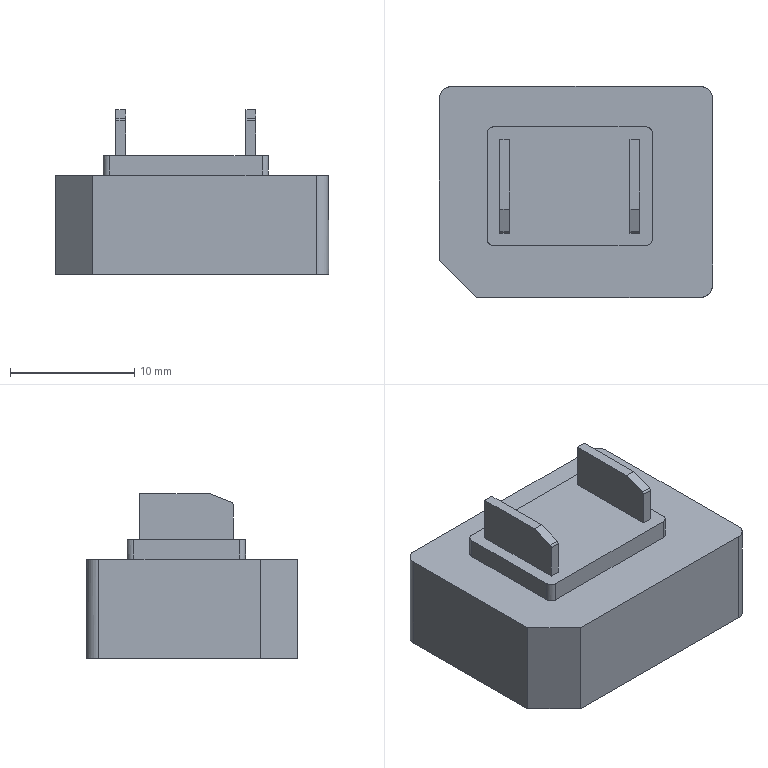NC program | PowerMill | posted by the shop | part box 22 x 17 x 13.286 mm
Lines 1 to 1591 of 53717:
%
G40 G49 G17 G80
( TOOL ID   D10C_1_1 )
( TOOL DIA. 10. TIP RAD 0 LENGTH 68.72 )
( Z = -.055 )
T1 M6
T2
G91 G28 Z0
G0 G90 G54
M08
S8000 M3
G0 X0 Y0 M8
G43 Z10.2 H1
X13.8 Y11.3
Z1.145
G1 Z-.055 F6000
X-13.8 F10000
Y5.65
X13.8
Y0
X-13.8
Y-5.65
X13.8
Y-11.3
X-13.8
X-18.8
G0 Z10.2
X-.5 Y.458
Z9.895
X19.223 Y5.979
Z.727
G1 Z-.473 F6000
X18.695 F10000
G3 X13.948 Y1.231 I0 J-4.748
G1 Y-11.112
G2 X12.948 Y-12.112 I-1. J0
G1 X-13.947
G2 X-14.947 Y-11.112 I0 J1.
G1 Y12.027
G2 X-13.947 Y13.027 I1. J0
G1 X12.948
G2 X13.948 Y12.027 I0 J-1.
G1 Y1.231
X10.448
Y-1.863
X10.42 Y-2.636
X10.293 Y-3.41
X10.051 Y-4.183
X9.942 Y-4.443
X9.671 Y-4.956
X9.168 Y-5.668
X8.395 Y-6.418
X7.621 Y-6.924
X6.796 Y-7.277
X6.075 Y-7.462
X5.301 Y-7.542
X4.528 Y-7.544
X3.754 Y-7.511
X2.981 Y-7.364
X2.207 Y-7.089
X1.434 Y-6.662
X1.212 Y-6.503
X.661 Y-6.033
X.378 Y-5.73
X-.099 Y-5.088
G3 X-.901 Y-5.088 I-.401 J-.298
G1 X-1.379 Y-5.73
X-1.66 Y-6.032
X-2.213 Y-6.503
X-2.433 Y-6.661
X-3.206 Y-7.088
X-3.98 Y-7.364
X-4.753 Y-7.511
X-5.527 Y-7.544
X-6.3 Y-7.542
X-7.074 Y-7.462
X-7.847 Y-7.261
X-8.62 Y-6.924
X-9.394 Y-6.418
X-10.114 Y-5.73
X-10.673 Y-4.956
X-10.941 Y-4.445
X-11.051 Y-4.183
X-11.294 Y-3.41
X-11.42 Y-2.636
X-11.448 Y-1.863
X-11.447 Y4.325
X-11.376 Y5.098
X-11.187 Y5.871
X-10.941 Y6.492
X-10.381 Y7.418
X-10.167 Y7.684
X-9.667 Y8.192
X-9.394 Y8.419
X-8.62 Y8.917
X-7.847 Y9.249
X-7.074 Y9.447
X-6.3 Y9.527
X-5.527 Y9.529
X-4.753 Y9.496
X-3.98 Y9.35
X-3.206 Y9.079
X-2.966 Y8.965
X-2.433 Y8.658
X-1.825 Y8.192
X-1.66 Y8.039
X-1.111 Y7.418
X-.91 Y7.13
G3 X-.09 Y7.13 I.41 J.286
G1 X.111 Y7.418
X.661 Y8.04
X.825 Y8.192
X1.434 Y8.658
X1.966 Y8.965
X2.207 Y9.079
X2.981 Y9.351
X3.754 Y9.496
X4.528 Y9.529
X5.301 Y9.527
X6.075 Y9.447
X6.848 Y9.249
X7.527 Y8.965
X8.395 Y8.418
X8.667 Y8.192
X9.168 Y7.683
X9.381 Y7.418
X9.865 Y6.645
X10.187 Y5.871
X10.376 Y5.098
X10.447 Y4.325
X10.448 Y1.231
X13.948
G0 Z3.36
G1 X19.223 Y5.979
G0 Z.36
G1 Z-.84 F6000
X18.695 F10000
G3 X13.948 Y1.231 I0 J-4.748
G1 Y-11.112
G2 X12.948 Y-12.112 I-1. J0
G1 X-13.947
G2 X-14.947 Y-11.112 I0 J1.
G1 Y12.027
G2 X-13.947 Y13.027 I1. J0
G1 X12.948
G2 X13.948 Y12.027 I0 J-1.
G1 Y2.497
X10.447 Y2.496
X10.448 Y.668
Y-1.863
Y-1.864
Y-2.636
X10.432 Y-3.41
X10.325 Y-4.183
X10.107 Y-4.956
X9.942 Y-5.36
X9.755 Y-5.73
X9.168 Y-6.582
X8.453 Y-7.277
X7.621 Y-7.834
X7.162 Y-8.05
X6.848 Y-8.161
X6.075 Y-8.362
X5.301 Y-8.448
X4.528 Y-8.45
X3.754 Y-8.413
X2.981 Y-8.27
X2.333 Y-8.05
X1.434 Y-7.566
X1.041 Y-7.277
X.661 Y-6.945
X.262 Y-6.503
X-.095 Y-6.009
G3 X-.905 Y-6.008 I-.405 J-.293
G1 X-1.264 Y-6.503
X-1.66 Y-6.944
X-2.03 Y-7.277
X-2.433 Y-7.565
X-3.206 Y-7.997
X-3.98 Y-8.27
X-4.753 Y-8.413
X-5.527 Y-8.45
X-6.3 Y-8.448
X-7.074 Y-8.362
X-7.847 Y-8.161
X-8.159 Y-8.05
X-8.62 Y-7.834
X-9.462 Y-7.277
X-10.167 Y-6.584
X-10.756 Y-5.73
X-10.941 Y-5.363
X-11.107 Y-4.956
X-11.326 Y-4.183
X-11.433 Y-3.41
X-11.448 Y-2.636
Y-1.864
Y-1.863
Y.686
X-11.447 Y4.325
X-11.376 Y5.098
X-11.187 Y5.871
X-10.941 Y6.492
X-10.381 Y7.418
X-10.167 Y7.684
X-9.667 Y8.192
X-9.394 Y8.419
X-8.62 Y8.917
X-7.847 Y9.249
X-7.074 Y9.447
X-6.3 Y9.527
X-5.527 Y9.529
X-4.753 Y9.496
X-3.98 Y9.35
X-3.206 Y9.079
X-2.966 Y8.965
X-2.433 Y8.658
X-1.825 Y8.192
X-1.66 Y8.039
X-1.111 Y7.418
X-.91 Y7.13
G3 X-.09 Y7.13 I.41 J.286
G1 X.111 Y7.418
X.661 Y8.04
X.825 Y8.192
X1.434 Y8.658
X1.966 Y8.965
X2.207 Y9.079
X2.981 Y9.351
X3.754 Y9.496
X4.528 Y9.529
X5.301 Y9.527
X6.075 Y9.447
X6.848 Y9.249
X7.527 Y8.965
X8.395 Y8.418
X8.667 Y8.192
X9.168 Y7.683
X9.381 Y7.418
X9.865 Y6.645
X10.187 Y5.871
X10.376 Y5.098
X10.447 Y4.325
Y2.496
X13.948 Y2.497
Y1.231
G0 Z2.992
G1 X19.223 Y5.979
G0 Z-.008
G1 Z-1.208 F6000
X18.695 F10000
G3 X13.948 Y1.231 I0 J-4.748
G1 Y-11.112
G2 X12.948 Y-12.112 I-1. J0
G1 X-13.947
G2 X-14.947 Y-11.112 I0 J1.
G1 Y12.027
G2 X-13.947 Y13.027 I1. J0
G1 X12.948
G2 X13.948 Y12.027 I0 J-1.
G1 Y2.268
X10.447
X10.448 Y.668
Y-1.863
Y-1.864
Y-2.636
X10.447 Y-2.677
Y-3.41
X10.376 Y-4.183
X10.187 Y-4.956
X9.942 Y-5.575
X9.381 Y-6.503
X9.168 Y-6.768
X8.668 Y-7.277
X8.395 Y-7.504
X7.528 Y-8.05
X6.848 Y-8.334
X6.075 Y-8.533
X5.301 Y-8.612
X4.528 Y-8.615
X3.754 Y-8.582
X2.981 Y-8.436
X2.207 Y-8.165
X1.964 Y-8.05
X1.434 Y-7.744
X.824 Y-7.277
X.661 Y-7.125
X.111 Y-6.503
X-.09 Y-6.216
G3 X-.91 Y-6.216 I-.41 J-.286
G1 X-1.111 Y-6.503
X-1.66 Y-7.124
X-1.824 Y-7.277
X-2.433 Y-7.744
X-2.964 Y-8.05
X-3.206 Y-8.164
X-3.98 Y-8.436
X-4.753 Y-8.582
X-5.527 Y-8.615
X-6.3 Y-8.612
X-7.074 Y-8.533
X-7.847 Y-8.335
X-8.528 Y-8.05
X-9.394 Y-7.504
X-9.668 Y-7.277
X-10.167 Y-6.769
X-10.381 Y-6.503
X-10.866 Y-5.73
X-11.187 Y-4.956
X-11.376 Y-4.183
X-11.447 Y-3.41
Y-2.678
X-11.448 Y-2.636
Y-1.864
Y-1.863
Y.686
X-11.447 Y3.847
Y4.325
X-11.376 Y5.098
X-11.187 Y5.871
X-10.941 Y6.492
X-10.381 Y7.418
X-10.167 Y7.684
X-9.667 Y8.192
X-9.394 Y8.419
X-8.62 Y8.917
X-7.847 Y9.249
X-7.074 Y9.447
X-6.3 Y9.527
X-5.527 Y9.529
X-4.753 Y9.496
X-3.98 Y9.35
X-3.206 Y9.079
X-2.966 Y8.965
X-2.433 Y8.658
X-1.825 Y8.192
X-1.66 Y8.039
X-1.111 Y7.418
X-.91 Y7.13
G3 X-.09 Y7.13 I.41 J.286
G1 X.111 Y7.418
X.661 Y8.04
X.825 Y8.192
X1.434 Y8.658
X1.966 Y8.965
X2.207 Y9.079
X2.981 Y9.351
X3.754 Y9.496
X4.528 Y9.529
X5.301 Y9.527
X6.075 Y9.447
X6.848 Y9.249
X7.527 Y8.965
X8.395 Y8.418
X8.667 Y8.192
X9.168 Y7.683
X9.381 Y7.418
X9.865 Y6.645
X10.187 Y5.871
X10.376 Y5.098
X10.447 Y4.325
Y3.867
Y2.268
X13.948
Y1.231
G0 Z2.625
G1 X19.223 Y5.979
G0 Z-.375
G1 Z-1.575 F6000
X18.695 F10000
G3 X13.948 Y1.231 I0 J-4.748
G1 Y-11.112
G2 X12.948 Y-12.112 I-1. J0
G1 X-13.947
G2 X-14.947 Y-11.112 I0 J1.
G1 Y12.027
G2 X-13.947 Y13.027 I1. J0
G1 X12.948
G2 X13.948 Y12.027 I0 J-1.
G1 Y2.038
X10.447
X10.448 Y.668
Y-1.863
Y-1.864
Y-2.636
X10.447 Y-2.674
Y-3.41
X10.376 Y-4.183
X10.187 Y-4.956
X9.942 Y-5.575
X9.381 Y-6.503
X9.168 Y-6.768
X8.668 Y-7.277
X8.395 Y-7.504
X7.528 Y-8.05
X6.848 Y-8.334
X6.075 Y-8.533
X5.301 Y-8.612
X4.528 Y-8.615
X3.754 Y-8.582
X2.981 Y-8.436
X2.207 Y-8.165
X1.964 Y-8.05
X1.434 Y-7.744
X.824 Y-7.277
X.661 Y-7.125
X.111 Y-6.503
X-.09 Y-6.216
G3 X-.91 Y-6.216 I-.41 J-.286
G1 X-1.111 Y-6.503
X-1.66 Y-7.124
X-1.824 Y-7.277
X-2.433 Y-7.744
X-2.964 Y-8.05
X-3.206 Y-8.164
X-3.98 Y-8.436
X-4.753 Y-8.582
X-5.527 Y-8.615
X-6.3 Y-8.612
X-7.074 Y-8.533
X-7.847 Y-8.335
X-8.528 Y-8.05
X-9.394 Y-7.504
X-9.668 Y-7.277
X-10.167 Y-6.769
X-10.381 Y-6.503
X-10.866 Y-5.73
X-11.187 Y-4.956
X-11.376 Y-4.183
X-11.447 Y-3.41
Y-2.674
X-11.448 Y-2.636
Y-1.864
Y-1.863
Y.686
X-11.447 Y3.367
Y4.325
X-11.376 Y5.098
X-11.187 Y5.871
X-10.941 Y6.492
X-10.381 Y7.418
X-10.167 Y7.684
X-9.667 Y8.192
X-9.394 Y8.419
X-8.62 Y8.917
X-7.847 Y9.249
X-7.074 Y9.447
X-6.3 Y9.527
X-5.527 Y9.529
X-4.753 Y9.496
X-3.98 Y9.35
X-3.206 Y9.079
X-2.966 Y8.965
X-2.433 Y8.658
X-1.825 Y8.192
X-1.66 Y8.039
X-1.111 Y7.418
X-.91 Y7.13
G3 X-.09 Y7.13 I.41 J.286
G1 X.111 Y7.418
X.661 Y8.04
X.825 Y8.192
X1.434 Y8.658
X1.966 Y8.965
X2.207 Y9.079
X2.981 Y9.351
X3.754 Y9.496
X4.528 Y9.529
X5.301 Y9.527
X6.075 Y9.447
X6.848 Y9.249
X7.527 Y8.965
X8.395 Y8.418
X8.667 Y8.192
X9.168 Y7.683
X9.381 Y7.418
X9.865 Y6.645
X10.187 Y5.871
X10.376 Y5.098
X10.447 Y4.325
Y3.408
Y2.038
X13.948
Y1.231
G0 Z2.257
G1 X19.223 Y5.979
G0 Z-.743
G1 Z-1.943 F6000
X18.695 F10000
G3 X13.948 Y1.231 I0 J-4.748
G1 Y-11.112
G2 X12.948 Y-12.112 I-1. J0
G1 X-13.947
G2 X-14.947 Y-11.112 I0 J1.
G1 Y-.588
X-11.448 Y-.589
Y.686
X-11.447 Y2.884
Y4.325
X-11.376 Y5.098
X-11.187 Y5.871
X-10.941 Y6.492
X-10.381 Y7.418
X-10.167 Y7.684
X-9.667 Y8.192
X-9.394 Y8.419
X-8.62 Y8.917
X-7.847 Y9.249
X-7.074 Y9.447
X-6.3 Y9.527
X-5.527 Y9.529
X-4.753 Y9.496
X-3.98 Y9.35
X-3.206 Y9.079
X-2.966 Y8.965
X-2.433 Y8.658
X-1.825 Y8.192
X-1.66 Y8.039
X-1.111 Y7.418
X-.91 Y7.13
G3 X-.09 Y7.13 I.41 J.286
G1 X.111 Y7.418
X.661 Y8.04
X.825 Y8.192
X1.434 Y8.658
X1.966 Y8.965
X2.207 Y9.079
X2.981 Y9.351
X3.754 Y9.496
X4.528 Y9.529
X5.301 Y9.527
X6.075 Y9.447
X6.848 Y9.249
X7.527 Y8.965
X8.395 Y8.418
X8.667 Y8.192
X9.168 Y7.683
X9.381 Y7.418
X9.865 Y6.645
X10.187 Y5.871
X10.376 Y5.098
X10.447 Y4.325
Y2.947
X10.448 Y.668
Y-1.863
Y-1.864
Y-2.636
X10.447 Y-2.671
Y-3.41
X10.376 Y-4.183
X10.187 Y-4.956
X9.942 Y-5.575
X9.381 Y-6.503
X9.168 Y-6.768
X8.668 Y-7.277
X8.395 Y-7.504
X7.528 Y-8.05
X6.848 Y-8.335
X6.075 Y-8.533
X5.301 Y-8.612
X4.528 Y-8.615
X3.754 Y-8.582
X2.981 Y-8.436
X2.207 Y-8.165
X1.964 Y-8.05
X1.434 Y-7.744
X.824 Y-7.277
X.661 Y-7.125
X.111 Y-6.503
X-.09 Y-6.216
G3 X-.91 Y-6.216 I-.41 J-.286
G1 X-1.111 Y-6.503
X-1.66 Y-7.124
X-1.824 Y-7.277
X-2.433 Y-7.744
X-2.964 Y-8.05
X-3.206 Y-8.164
X-3.98 Y-8.436
X-4.753 Y-8.582
X-5.527 Y-8.615
X-6.3 Y-8.612
X-7.074 Y-8.533
X-7.847 Y-8.335
X-8.528 Y-8.05
X-9.394 Y-7.504
X-9.668 Y-7.277
X-10.167 Y-6.769
X-10.382 Y-6.503
X-10.866 Y-5.73
X-11.187 Y-4.956
X-11.376 Y-4.183
X-11.447 Y-3.41
Y-2.671
X-11.448 Y-2.636
Y-1.864
Y-1.863
Y-.589
X-14.947 Y-.588
Y12.027
G2 X-13.947 Y13.027 I1. J0
G1 X12.948
G2 X13.948 Y12.027 I0 J-1.
G1 Y1.231
G0 Z1.89
G1 X19.223 Y5.979
G0 Z-1.11
G1 Z-2.31 F6000
X18.695 F10000
G3 X13.948 Y1.231 I0 J-4.748
G1 Y-11.112
G2 X12.948 Y-12.112 I-1. J0
G1 X-13.947
G2 X-14.947 Y-11.112 I0 J1.
G1 Y-.588
X-11.448 Y-.589
X-11.447 Y.686
Y2.398
Y4.325
X-11.376 Y5.098
X-11.187 Y5.871
X-10.941 Y6.492
X-10.381 Y7.418
X-10.167 Y7.684
X-9.667 Y8.192
X-9.394 Y8.419
X-8.62 Y8.917
X-7.847 Y9.249
X-7.074 Y9.447
X-6.3 Y9.527
X-5.527 Y9.529
X-4.753 Y9.496
X-3.98 Y9.35
X-3.206 Y9.079
X-2.966 Y8.965
X-2.433 Y8.658
X-1.825 Y8.192
X-1.66 Y8.039
X-1.111 Y7.418
X-.91 Y7.13
G3 X-.09 Y7.13 I.41 J.286
G1 X.111 Y7.418
X.661 Y8.04
X.825 Y8.192
X1.434 Y8.658
X1.966 Y8.965
X2.207 Y9.079
X2.981 Y9.351
X3.754 Y9.496
X4.528 Y9.529
X5.301 Y9.527
X6.075 Y9.447
X6.848 Y9.249
X7.527 Y8.965
X8.395 Y8.418
X8.667 Y8.192
X9.168 Y7.683
X9.381 Y7.418
X9.865 Y6.645
X10.187 Y5.871
X10.376 Y5.098
X10.447 Y4.325
Y2.484
Y.668
X10.448 Y-1.863
Y-1.864
Y-2.636
X10.447 Y-2.668
Y-3.41
X10.376 Y-4.183
X10.187 Y-4.956
X9.942 Y-5.575
X9.381 Y-6.503
X9.168 Y-6.768
X8.668 Y-7.277
X8.395 Y-7.504
X7.528 Y-8.05
X6.848 Y-8.335
X6.075 Y-8.533
X5.301 Y-8.612
X4.528 Y-8.615
X3.754 Y-8.582
X2.981 Y-8.436
X2.207 Y-8.165
X1.964 Y-8.05
X1.434 Y-7.744
X.824 Y-7.277
X.661 Y-7.125
X.111 Y-6.503
X-.09 Y-6.216
G3 X-.91 Y-6.216 I-.41 J-.286
G1 X-1.111 Y-6.503
X-1.66 Y-7.124
X-1.824 Y-7.277
X-2.433 Y-7.744
X-2.964 Y-8.05
X-3.206 Y-8.164
X-3.98 Y-8.436
X-4.753 Y-8.582
X-5.527 Y-8.615
X-6.3 Y-8.612
X-7.074 Y-8.533
X-7.847 Y-8.335
X-8.528 Y-8.05
X-9.394 Y-7.504
X-9.668 Y-7.277
X-10.167 Y-6.769
X-10.382 Y-6.503
X-10.866 Y-5.73
X-11.187 Y-4.956
X-11.376 Y-4.183
X-11.447 Y-3.41
Y-2.668
X-11.448 Y-2.636
Y-1.864
Y-1.863
Y-.589
X-14.947 Y-.588
Y12.027
G2 X-13.947 Y13.027 I1. J0
G1 X12.948
G2 X13.948 Y12.027 I0 J-1.
G1 Y1.231
G0 Z1.522
G1 X19.223 Y5.979
G0 Z-1.478
G1 Z-2.678 F6000
X18.695 F10000
G3 X13.948 Y1.231 I0 J-4.748
G1 Y-11.112
G2 X12.948 Y-12.112 I-1. J0
G1 X-13.947
G2 X-14.947 Y-11.112 I0 J1.
G1 Y-.588
X-11.448 Y-.589
X-11.447 Y.686
Y1.909
Y4.325
X-11.376 Y5.098
X-11.187 Y5.871
X-10.941 Y6.492
X-10.381 Y7.418
X-10.167 Y7.684
X-9.667 Y8.192
X-9.394 Y8.419
X-8.62 Y8.917
X-7.847 Y9.249
X-7.074 Y9.447
X-6.3 Y9.527
X-5.527 Y9.529
X-4.753 Y9.496
X-3.98 Y9.35
X-3.206 Y9.079
X-2.966 Y8.965
X-2.433 Y8.658
X-1.825 Y8.192
X-1.66 Y8.039
X-1.111 Y7.418
X-.91 Y7.13
G3 X-.09 Y7.13 I.41 J.286
G1 X.111 Y7.418
X.661 Y8.04
X.825 Y8.192
X1.434 Y8.658
X1.966 Y8.965
X2.207 Y9.079
X2.981 Y9.351
X3.754 Y9.496
X4.528 Y9.529
X5.301 Y9.527
X6.075 Y9.447
X6.848 Y9.249
X7.527 Y8.965
X8.395 Y8.418
X8.667 Y8.192
X9.168 Y7.683
X9.381 Y7.418
X9.865 Y6.645
X10.187 Y5.871
X10.376 Y5.098
X10.447 Y4.325
Y2.014
Y.668
X10.448 Y-1.863
Y-1.864
Y-2.636
X10.447 Y-2.665
Y-3.41
X10.376 Y-4.183
X10.187 Y-4.956
X9.942 Y-5.575
X9.381 Y-6.503
X9.168 Y-6.768
X8.668 Y-7.277
X8.395 Y-7.504
X7.528 Y-8.05
X6.848 Y-8.335
X6.075 Y-8.533
X5.301 Y-8.612
X4.528 Y-8.615
X3.754 Y-8.582
X2.981 Y-8.436
X2.207 Y-8.165
X1.964 Y-8.05
X1.434 Y-7.744
X.824 Y-7.277
X.661 Y-7.125
X.111 Y-6.503
X-.09 Y-6.216
G3 X-.91 Y-6.216 I-.41 J-.286
G1 X-1.111 Y-6.503
X-1.66 Y-7.124
X-1.824 Y-7.277
X-2.433 Y-7.744
X-2.964 Y-8.05
X-3.206 Y-8.164
X-3.98 Y-8.436
X-4.753 Y-8.582
X-5.527 Y-8.615
X-6.3 Y-8.612
X-7.074 Y-8.533
X-7.847 Y-8.335
X-8.528 Y-8.05
X-9.394 Y-7.504
X-9.668 Y-7.277
X-10.167 Y-6.769
X-10.382 Y-6.503
X-10.866 Y-5.73
X-11.187 Y-4.956
X-11.376 Y-4.183
X-11.447 Y-3.41
Y-2.665
X-11.448 Y-2.636
Y-1.864
Y-1.863
Y-.589
X-14.947 Y-.588
Y12.027
G2 X-13.947 Y13.027 I1. J0
G1 X12.948
G2 X13.948 Y12.027 I0 J-1.
G1 Y1.231
G0 Z1.155
G1 X19.223 Y5.979
G0 Z-1.845
G1 Z-3.045 F6000
X18.695 F10000
G3 X13.948 Y1.231 I0 J-4.748
G1 Y-11.112
G2 X12.948 Y-12.112 I-1. J0
G1 X-13.947
G2 X-14.947 Y-11.112 I0 J1.
G1 Y2.871
X-11.447
Y4.325
X-11.376 Y5.098
X-11.187 Y5.871
X-10.941 Y6.492
X-10.381 Y7.418
X-10.167 Y7.684
X-9.667 Y8.192
X-9.394 Y8.419
X-8.62 Y8.917
X-7.847 Y9.249
X-7.074 Y9.447
X-6.3 Y9.527
X-5.527 Y9.529
X-4.753 Y9.496
X-3.98 Y9.35
X-3.206 Y9.079
X-2.966 Y8.965
X-2.433 Y8.658
X-1.825 Y8.192
X-1.66 Y8.039
X-1.111 Y7.418
X-.91 Y7.13
G3 X-.09 Y7.13 I.41 J.286
G1 X.111 Y7.418
X.661 Y8.04
X.825 Y8.192
X1.434 Y8.659
X1.966 Y8.965
X2.207 Y9.079
X2.981 Y9.351
X3.754 Y9.496
X4.528 Y9.529
X5.301 Y9.527
X6.075 Y9.447
X6.848 Y9.249
X7.527 Y8.965
X8.395 Y8.418
X8.667 Y8.192
X9.168 Y7.683
X9.381 Y7.418
X9.865 Y6.645
X10.187 Y5.871
X10.376 Y5.098
X10.447 Y4.325
Y1.548
Y.668
X10.448 Y-1.863
Y-1.864
Y-2.636
X10.447 Y-2.662
Y-3.41
X10.376 Y-4.183
X10.187 Y-4.956
X9.942 Y-5.575
X9.381 Y-6.503
X9.168 Y-6.768
X8.668 Y-7.277
X8.395 Y-7.504
X7.528 Y-8.05
X6.848 Y-8.335
X6.075 Y-8.533
X5.301 Y-8.612
X4.528 Y-8.615
X3.754 Y-8.582
X2.981 Y-8.436
X2.207 Y-8.165
X1.964 Y-8.05
X1.434 Y-7.744
X.824 Y-7.277
X.661 Y-7.125
X.111 Y-6.503
X-.09 Y-6.216
G3 X-.91 Y-6.216 I-.41 J-.286
G1 X-1.111 Y-6.503
X-1.66 Y-7.124
X-1.824 Y-7.277
X-2.433 Y-7.744
X-2.964 Y-8.05
X-3.206 Y-8.164
X-3.98 Y-8.436
X-4.753 Y-8.582
X-5.527 Y-8.615
X-6.3 Y-8.612
X-7.074 Y-8.533
X-7.847 Y-8.335
X-8.528 Y-8.05
X-9.394 Y-7.504
X-9.668 Y-7.277
X-10.167 Y-6.769
X-10.382 Y-6.503
X-10.866 Y-5.73
X-11.187 Y-4.956
X-11.376 Y-4.183
X-11.447 Y-3.41
Y-2.662
X-11.448 Y-2.636
Y-1.864
Y-1.863
X-11.447 Y.686
Y1.417
Y2.871
X-14.947
Y12.027
G2 X-13.947 Y13.027 I1. J0
G1 X12.948
G2 X13.948 Y12.027 I0 J-1.
G1 Y1.231
G0 Z.787
G1 X19.223 Y5.979
G0 Z-2.213
G1 Z-3.413 F6000
X18.695 F10000
G3 X13.948 Y1.231 I0 J-4.748
G1 Y-11.112
G2 X12.948 Y-12.112 I-1. J0
G1 X-13.947
G2 X-14.947 Y-11.112 I0 J1.
G1 Y2.647
X-11.447
Y4.325
X-11.376 Y5.098
X-11.187 Y5.871
X-10.941 Y6.492
X-10.381 Y7.418
X-10.167 Y7.684
X-9.667 Y8.192
X-9.394 Y8.419
X-8.62 Y8.917
X-7.847 Y9.249
X-7.074 Y9.447
X-6.3 Y9.527
X-5.527 Y9.529
X-4.753 Y9.496
X-3.98 Y9.35
X-3.206 Y9.079
X-2.966 Y8.965
X-2.433 Y8.658
X-1.825 Y8.192
X-1.66 Y8.039
X-1.111 Y7.418
X-.91 Y7.13
G3 X-.09 Y7.13 I.41 J.286
G1 X.111 Y7.418
X.661 Y8.04
X.825 Y8.192
X1.434 Y8.659
X1.966 Y8.965
X2.207 Y9.079
X2.981 Y9.351
X3.754 Y9.496
X4.528 Y9.529
X5.301 Y9.527
X6.075 Y9.447
X6.848 Y9.249
X7.527 Y8.965
X8.395 Y8.418
X8.667 Y8.192
X9.168 Y7.683
X9.381 Y7.418
X9.865 Y6.645
X10.187 Y5.871
X10.376 Y5.098
X10.447 Y4.325
Y1.081
Y.668
X10.448 Y-1.863
Y-1.864
Y-2.636
X10.447 Y-2.659
Y-3.41
X10.376 Y-4.183
X10.187 Y-4.956
X9.942 Y-5.575
X9.381 Y-6.503
X9.168 Y-6.768
X8.668 Y-7.277
X8.395 Y-7.504
X7.528 Y-8.05
X6.848 Y-8.335
X6.075 Y-8.533
X5.301 Y-8.612
X4.528 Y-8.615
X3.754 Y-8.582
X2.981 Y-8.436
X2.207 Y-8.165
X1.964 Y-8.05
X1.434 Y-7.744
X.824 Y-7.277
X.661 Y-7.125
X.111 Y-6.503
X-.09 Y-6.216
G3 X-.91 Y-6.216 I-.41 J-.286
G1 X-1.111 Y-6.503
X-1.66 Y-7.124
X-1.824 Y-7.277
X-2.433 Y-7.744
X-2.964 Y-8.05
X-3.206 Y-8.164
X-3.98 Y-8.436
X-4.753 Y-8.582
X-5.527 Y-8.615
X-6.3 Y-8.612
X-7.074 Y-8.533
X-7.847 Y-8.335
X-8.528 Y-8.05
X-9.394 Y-7.504
X-9.668 Y-7.277
X-10.167 Y-6.769
X-10.382 Y-6.503
X-10.866 Y-5.73
X-11.187 Y-4.956
X-11.376 Y-4.183
X-11.447 Y-3.41
Y-2.658
X-11.448 Y-2.636
Y-1.864
Y-1.863
X-11.447 Y.969
Y2.647
X-14.947
Y12.027
G2 X-13.947 Y13.027 I1. J0
G1 X12.948
G2 X13.948 Y12.027 I0 J-1.
G1 Y1.231
G0 Z.42
G1 X19.223 Y5.979
G0 Z-2.58
G1 Z-3.78 F6000
X18.695 F10000
G3 X13.948 Y1.231 I0 J-4.748
G1 Y-11.112
G2 X12.948 Y-12.112 I-1. J0
G1 X-13.947
G2 X-14.947 Y-11.112 I0 J1.
G1 Y2.421
X-11.447
Y4.325
X-11.376 Y5.098
X-11.187 Y5.871
X-10.941 Y6.492
X-10.381 Y7.418
X-10.167 Y7.684
X-9.667 Y8.192
X-9.394 Y8.419
X-8.62 Y8.917
X-7.847 Y9.249
X-7.074 Y9.447
X-6.3 Y9.527
X-5.527 Y9.529
X-4.753 Y9.496
X-3.98 Y9.35
X-3.206 Y9.079
X-2.966 Y8.965
X-2.433 Y8.658
X-1.825 Y8.192
X-1.66 Y8.039
X-1.111 Y7.418
X-.91 Y7.13
G3 X-.09 Y7.13 I.41 J.286
G1 X.111 Y7.418
X.661 Y8.04
X.825 Y8.192
X1.434 Y8.659
X1.966 Y8.965
X2.207 Y9.079
X2.981 Y9.351
X3.754 Y9.496
X4.528 Y9.529
X5.301 Y9.527
X6.075 Y9.447
X6.848 Y9.249
X7.527 Y8.965
X8.395 Y8.418
X8.667 Y8.192
X9.168 Y7.683
X9.381 Y7.418
X9.865 Y6.645
X10.187 Y5.871
X10.376 Y5.098
X10.447 Y4.325
Y.658
X10.448 Y-1.863
Y-1.864
Y-2.636
X10.447 Y-2.656
Y-3.41
X10.376 Y-4.183
X10.187 Y-4.956
X9.942 Y-5.575
X9.382 Y-6.503
X9.168 Y-6.768
X8.668 Y-7.277
X8.395 Y-7.504
X7.528 Y-8.05
X6.848 Y-8.335
X6.075 Y-8.533
X5.301 Y-8.612
X4.528 Y-8.615
X3.754 Y-8.582
X2.981 Y-8.436
X2.207 Y-8.165
X1.964 Y-8.05
X1.434 Y-7.744
X.824 Y-7.277
X.661 Y-7.125
X.111 Y-6.503
X-.09 Y-6.216
G3 X-.91 Y-6.216 I-.41 J-.286
G1 X-1.111 Y-6.503
X-1.66 Y-7.124
X-1.824 Y-7.277
X-2.433 Y-7.744
X-2.964 Y-8.05
X-3.206 Y-8.164
X-3.98 Y-8.436
X-4.753 Y-8.582
X-5.527 Y-8.615
X-6.3 Y-8.612
X-7.074 Y-8.533
X-7.847 Y-8.335
X-8.528 Y-8.05
X-9.394 Y-7.504
X-9.668 Y-7.277
X-10.167 Y-6.769
X-10.382 Y-6.503
X-10.866 Y-5.73
X-11.187 Y-4.956
X-11.376 Y-4.183
X-11.447 Y-3.41
Y-2.655
X-11.448 Y-2.636
Y-1.864
Y-1.863
X-11.447 Y.518
Y2.421
X-14.947
Y12.027
G2 X-13.947 Y13.027 I1. J0
G1 X12.948
G2 X13.948 Y12.027 I0 J-1.
G1 Y1.231
G0 Z.04
G1 X19.223 Y5.979
G0 Z-2.96
G1 Z-4.16 F6000
X18.695 F10000
G3 X13.948 Y1.231 I0 J-4.748
G1 Y-11.112
G2 X12.948 Y-12.112 I-1. J0
G1 X-13.947
G2 X-14.947 Y-11.112 I0 J1.
G1 Y12.027
G2 X-13.947 Y13.027 I1. J0
G1 X-.499
X-.5 Y10.529
X5.301
X6.07 Y10.512
X6.848 Y10.401
X7.621 Y10.182
X8.395 Y9.834
X9.168 Y9.338
X9.609 Y8.965
X9.942 Y8.627
X10.301 Y8.192
X10.715 Y7.544
X11.122 Y6.645
X11.332 Y5.871
X11.435 Y5.098
X11.448 Y4.325
Y-3.41
X11.435 Y-4.183
X11.332 Y-4.956
X11.122 Y-5.73
X10.785 Y-6.503
X10.301 Y-7.277
X9.942 Y-7.713
X9.61 Y-8.05
X9.168 Y-8.424
X8.567 Y-8.824
X7.621 Y-9.268
X6.848 Y-9.487
X6.079 Y-9.597
X5.301 Y-9.615
X-6.3
X-7.074 Y-9.597
X-7.847 Y-9.487
X-8.62 Y-9.268
X-9.394 Y-8.92
X-10.167 Y-8.424
X-10.61 Y-8.05
X-10.941 Y-7.714
X-11.301 Y-7.277
X-11.714 Y-6.631
X-12.122 Y-5.73
X-12.332 Y-4.956
X-12.435 Y-4.183
X-12.448 Y-3.41
Y4.325
X-12.435 Y5.098
X-12.332 Y5.871
X-12.122 Y6.645
X-11.784 Y7.418
X-11.301 Y8.192
X-10.941 Y8.628
X-10.609 Y8.965
X-10.167 Y9.339
X-9.566 Y9.739
X-8.62 Y10.183
X-7.847 Y10.401
X-7.074 Y10.512
X-6.3 Y10.529
X-.5
X-.499 Y13.027
X12.948
G2 X13.948 Y12.027 I0 J-1.
G1 Y1.231
G0 Z-.34
G1 X19.223 Y5.979
G0 Z-3.34
G1 Z-4.54 F6000
X18.695 F10000
G3 X13.948 Y1.231 I0 J-4.748
G1 Y-11.112
G2 X12.948 Y-12.112 I-1. J0
G1 X-13.947
G2 X-14.947 Y-11.112 I0 J1.
G1 Y12.027
G2 X-13.947 Y13.027 I1. J0
G1 X-.499
X-.5 Y10.529
X5.301
X6.07 Y10.512
X6.848 Y10.401
X7.621 Y10.182
X8.395 Y9.834
X9.168 Y9.338
X9.609 Y8.965
X9.942 Y8.627
X10.301 Y8.192
X10.715 Y7.544
X11.122 Y6.645
X11.332 Y5.871
X11.435 Y5.098
X11.448 Y4.325
Y-3.41
X11.435 Y-4.183
X11.332 Y-4.956
X11.122 Y-5.73
X10.785 Y-6.503
X10.301 Y-7.277
X9.942 Y-7.713
X9.61 Y-8.05
X9.168 Y-8.424
X8.567 Y-8.824
X7.621 Y-9.268
X6.848 Y-9.487
X6.079 Y-9.597
X5.301 Y-9.615
X-6.3
X-7.074 Y-9.597
X-7.847 Y-9.487
X-8.62 Y-9.268
X-9.394 Y-8.92
X-10.167 Y-8.425
X-10.61 Y-8.05
X-10.941 Y-7.714
X-11.301 Y-7.277
X-11.714 Y-6.631
X-12.122 Y-5.73
X-12.332 Y-4.956
X-12.435 Y-4.183
X-12.448 Y-3.41
Y4.325
X-12.435 Y5.098
X-12.332 Y5.871
X-12.122 Y6.645
X-11.784 Y7.418
X-11.301 Y8.192
X-10.941 Y8.628
X-10.609 Y8.965
X-10.167 Y9.339
X-9.566 Y9.739
X-8.62 Y10.183
X-7.847 Y10.401
X-7.074 Y10.512
X-6.3 Y10.529
X-.5
X-.499 Y13.027
X12.948
G2 X13.948 Y12.027 I0 J-1.
G1 Y1.231
G0 Z-.72
G1 X19.223 Y5.979
G0 Z-3.72
G1 Z-4.92 F6000
X18.695 F10000
G3 X13.948 Y1.231 I0 J-4.748
G1 Y-11.112
G2 X12.948 Y-12.112 I-1. J0
G1 X-13.947
G2 X-14.947 Y-11.112 I0 J1.
G1 Y12.027
G2 X-13.947 Y13.027 I1. J0
G1 X-.499
X-.5 Y10.529
X5.301
X6.07 Y10.512
X6.848 Y10.401
X7.621 Y10.182
X8.395 Y9.834
X9.168 Y9.338
X9.609 Y8.965
X9.942 Y8.627
X10.301 Y8.192
X10.715 Y7.544
X11.122 Y6.645
X11.332 Y5.871
X11.435 Y5.098
X11.448 Y4.325
Y-3.41
X11.435 Y-4.183
X11.332 Y-4.956
X11.122 Y-5.73
X10.785 Y-6.503
X10.301 Y-7.277
X9.942 Y-7.713
X9.61 Y-8.05
X9.168 Y-8.424
X8.567 Y-8.824
X7.621 Y-9.268
X6.848 Y-9.487
X6.079 Y-9.597
X5.301 Y-9.615
X-6.3
X-7.074 Y-9.597
X-7.847 Y-9.487
X-8.62 Y-9.268
X-9.394 Y-8.92
X-10.167 Y-8.425
X-10.61 Y-8.05
X-10.941 Y-7.714
X-11.301 Y-7.277
X-11.714 Y-6.631
X-12.122 Y-5.73
X-12.332 Y-4.956
X-12.435 Y-4.183
X-12.448 Y-3.41
Y4.325
X-12.435 Y5.098
X-12.332 Y5.871
X-12.122 Y6.645
X-11.784 Y7.418
X-11.301 Y8.192
X-10.941 Y8.628
X-10.609 Y8.965
X-10.167 Y9.339
X-9.566 Y9.739
X-8.62 Y10.183
X-7.847 Y10.401
X-7.074 Y10.512
X-6.3 Y10.529
X-.5
X-.499 Y13.027
X12.948
G2 X13.948 Y12.027 I0 J-1.
G1 Y1.231
G0 Z-1.1
G1 X19.223 Y5.979
G0 Z-4.1
G1 Z-5.3 F6000
X18.695 F10000
G3 X13.948 Y1.231 I0 J-4.748
G1 Y-11.112
G2 X12.948 Y-12.112 I-1. J0
G1 X-13.947
G2 X-14.947 Y-11.112 I0 J1.
G1 Y12.027
G2 X-13.947 Y13.027 I1. J0
G1 X-.499
X-.5 Y10.529
X5.301
X6.07 Y10.512
X6.848 Y10.401
X7.621 Y10.182
X8.395 Y9.834
X9.168 Y9.338
X9.609 Y8.965
X9.942 Y8.627
X10.301 Y8.192
X10.715 Y7.544
X11.122 Y6.645
X11.332 Y5.871
X11.435 Y5.098
X11.448 Y4.325
Y-3.41
X11.435 Y-4.183
X11.332 Y-4.956
X11.122 Y-5.73
X10.785 Y-6.503
X10.301 Y-7.277
X9.942 Y-7.713
X9.61 Y-8.05
X9.168 Y-8.424
X8.567 Y-8.824
X7.621 Y-9.268
X6.848 Y-9.487
X6.079 Y-9.597
X5.301 Y-9.615
X-6.3
X-7.074 Y-9.598
X-7.847 Y-9.487
X-8.62 Y-9.268
X-9.394 Y-8.92
X-10.167 Y-8.425
X-10.61 Y-8.05
X-10.941 Y-7.714
X-11.301 Y-7.277
X-11.714 Y-6.631
X-12.122 Y-5.73
X-12.332 Y-4.956
X-12.435 Y-4.183
X-12.448 Y-3.41
Y4.325
X-12.435 Y5.098
X-12.332 Y5.871
X-12.122 Y6.645
X-11.784 Y7.418
X-11.301 Y8.192
X-10.941 Y8.628
X-10.609 Y8.965
X-10.167 Y9.339
X-9.566 Y9.739
X-8.62 Y10.183
X-7.847 Y10.401
X-7.074 Y10.512
X-6.3 Y10.529
X-.5
X-.499 Y13.027
X12.948
G2 X13.948 Y12.027 I0 J-1.
G1 Y1.231
G0 Z9.895
X-.5 Y.458
Z9.795
X14.54 Y-18.676
Z-4.478
G1 Z-5.678 F6000
G3 X12.383 Y-13.077 I-1.078 J2.799 F10000
G1 X11.875 Y-13.273
X11.102 Y-13.467
X10.328 Y-13.559
X-8.234 Y-13.565
X-9.007 Y-13.469
X-9.781 Y-13.247
X-10.18 Y-13.077
X-10.554 Y-12.88
X-11.327 Y-12.325
X-14.421 Y-9.249
X-15.195 Y-8.348
X-15.585 Y-7.663
X-15.876 Y-6.89
X-15.968 Y-6.512
X-16.032 Y-6.117
X-16.07 Y-5.343
X-16.061 Y7.805
X-15.968 Y8.594
X-15.781 Y9.352
X-15.47 Y10.125
X-15.195 Y10.639
X-15.028 Y10.899
X-14.408 Y11.672
X-13.519 Y12.446
X-12.874 Y12.846
X-12.033 Y13.219
X-11.327 Y13.423
X-10.554 Y13.54
X-9.781 Y13.57
X10.328 Y13.559
X11.102 Y13.467
X12.033 Y13.219
X12.649 Y12.959
X13.519 Y12.446
X14.196 Y11.886
X14.408 Y11.672
X15.028 Y10.899
X15.47 Y10.125
X15.781 Y9.352
X15.971 Y8.578
X16.061 Y7.805
X16.067 Y-7.663
X15.992 Y-8.437
X15.824 Y-9.21
X15.533 Y-9.984
X15.12 Y-10.757
X14.969 Y-10.986
X14.536 Y-11.531
X14.196 Y-11.886
X13.709 Y-12.304
X13.422 Y-12.513
X12.649 Y-12.959
X12.383 Y-13.077
X11.875 Y-13.273 Z-5.68
X11.102 Y-13.467 Z-5.683
X10.328 Y-13.559 Z-5.686
X-8.175 Y-13.567 Z-5.753
X-9.019 Y-13.466 Z-5.756
X-9.787 Y-13.245 Z-5.759
X-10.18 Y-13.077 Z-5.761
X-10.567 Y-12.872 Z-5.762
X-11.34 Y-12.314 Z-5.766
X-14.803 Y-8.853 Z-5.783
X-15.201 Y-8.338 Z-5.786
X-15.585 Y-7.663 Z-5.789
X-15.876 Y-6.89 Z-5.792
X-15.968 Y-6.512 Z-5.793
X-16.032 Y-6.117 Z-5.795
X-16.07 Y-5.343 Z-5.797
X-16.06 Y7.817 Z-5.845
X-15.968 Y8.594 Z-5.848
X-15.777 Y9.364 Z-5.851
X-15.466 Y10.134 Z-5.854
X-15.195 Y10.639 Z-5.856
X-14.724 Y11.31 Z-5.859
X-14.397 Y11.684 Z-5.861
X-14.035 Y12.032 Z-5.863
X-13.51 Y12.452 Z-5.865
X-12.874 Y12.846 Z-5.868
X-12.033 Y13.219 Z-5.871
X-11.327 Y13.423 Z-5.874
X-10.554 Y13.54 Z-5.877
X-9.781 Y13.57 Z-5.879
X10.341 Y13.559 Z-5.953
X11.114 Y13.465 Z-5.955
X12.033 Y13.219 Z-5.959
X12.661 Y12.953 Z-5.961
X13.519 Y12.446 Z-5.965
X14.196 Y11.886 Z-5.968